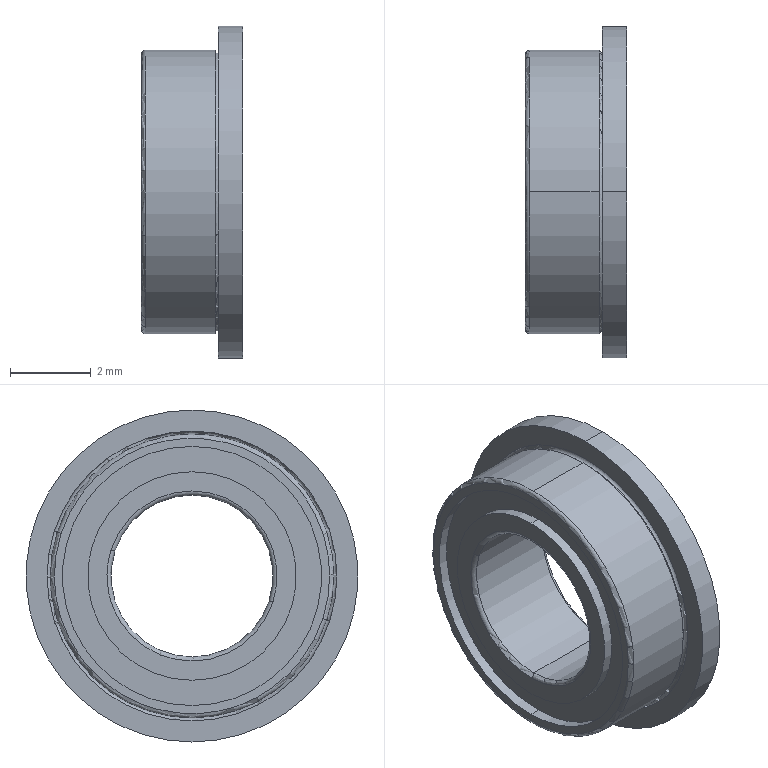Part | NX | features BREP 1 | 1 solid | 31 faces | box 2.5 x 8.2 x 8.2 mm | volume 67.176 mm3 | cylinder 14 | torus 10 | plane 7 | commonest cylinder face diameters 5.15 x4 6.4 x4 4 x2 7 x2 8.2 x2
STEP:
#1=CARTESIAN_POINT('',(1.9,-3.405,-1.106));
#2=VERTEX_POINT('',#1);
#3=CARTESIAN_POINT('',(1.9,-3.253,-1.057));
#4=VERTEX_POINT('',#3);
#5=CARTESIAN_POINT('',(1.9,-3.329,-1.082));
#6=DIRECTION('',(0.,0.309,-0.9511));
#7=DIRECTION('',(-1.,0.,0.));
#8=AXIS2_PLACEMENT_3D('',#5,#6,#7);
#9=CIRCLE('',#8,0.08);
#10=EDGE_CURVE('',#2,#4,#9,.F.);
#11=ORIENTED_EDGE('',*,*,#10,.T.);
#12=CARTESIAN_POINT('',(1.9,3.253,1.057));
#13=VERTEX_POINT('',#12);
#14=CARTESIAN_POINT('',(1.9,0.,0.));
#15=DIRECTION('',(1.,0.,0.));
#16=DIRECTION('',(0.,0.,-1.));
#17=AXIS2_PLACEMENT_3D('',#14,#15,#16);
#18=CIRCLE('',#17,3.42);
#19=EDGE_CURVE('',#4,#13,#18,.T.);
#20=ORIENTED_EDGE('',*,*,#19,.T.);
#21=CARTESIAN_POINT('',(1.9,3.405,1.106));
#22=VERTEX_POINT('',#21);
#23=CARTESIAN_POINT('',(1.9,3.329,1.082));
#24=DIRECTION('',(0.,-0.309,0.9511));
#25=DIRECTION('',(-1.,0.,0.));
#26=AXIS2_PLACEMENT_3D('',#23,#24,#25);
#27=CIRCLE('',#26,0.08);
#28=EDGE_CURVE('',#22,#13,#27,.F.);
#29=ORIENTED_EDGE('',*,*,#28,.F.);
#30=CARTESIAN_POINT('',(1.9,0.,0.));
#31=DIRECTION('',(1.,0.,0.));
#32=DIRECTION('',(0.,-0.9511,-0.309));
#33=AXIS2_PLACEMENT_3D('',#30,#31,#32);
#34=CIRCLE('',#33,3.58);
#35=EDGE_CURVE('',#2,#22,#34,.T.);
#36=ORIENTED_EDGE('',*,*,#35,.F.);
#37=EDGE_LOOP('',(#11,#20,#29,#36));
#38=FACE_BOUND('',#37,.T.);
#39=CARTESIAN_POINT('',(1.9,0.,0.));
#40=DIRECTION('',(1.,0.,0.));
#41=DIRECTION('',(0.,0.309,-0.9511));
#42=AXIS2_PLACEMENT_3D('',#39,#40,#41);
#43=TOROIDAL_SURFACE('',#42,3.5,0.08);
#44=ADVANCED_FACE('',(#38),#43,.F.);
#45=ORIENTED_EDGE('',*,*,#28,.T.);
#46=CARTESIAN_POINT('',(1.9,0.,0.));
#47=DIRECTION('',(1.,0.,0.));
#48=DIRECTION('',(0.,0.,-1.));
#49=AXIS2_PLACEMENT_3D('',#46,#47,#48);
#50=CIRCLE('',#49,3.42);
#51=EDGE_CURVE('',#13,#4,#50,.T.);
#52=ORIENTED_EDGE('',*,*,#51,.T.);
#53=ORIENTED_EDGE('',*,*,#10,.F.);
#54=CARTESIAN_POINT('',(1.9,0.,0.));
#55=DIRECTION('',(1.,0.,0.));
#56=DIRECTION('',(0.,0.,-1.));
#57=AXIS2_PLACEMENT_3D('',#54,#55,#56);
#58=CIRCLE('',#57,3.58);
#59=EDGE_CURVE('',#22,#2,#58,.T.);
#60=ORIENTED_EDGE('',*,*,#59,.F.);
#61=EDGE_LOOP('',(#45,#52,#53,#60));
#62=FACE_BOUND('',#61,.T.);
#63=CARTESIAN_POINT('',(1.9,0.,0.));
#64=DIRECTION('',(1.,0.,0.));
#65=DIRECTION('',(0.,-0.309,0.9511));
#66=AXIS2_PLACEMENT_3D('',#63,#64,#65);
#67=TOROIDAL_SURFACE('',#66,3.5,0.08);
#68=ADVANCED_FACE('',(#62),#67,.F.);
#69=CARTESIAN_POINT('',(0.,0.,2.575));
#70=VERTEX_POINT('',#69);
#71=CARTESIAN_POINT('',(0.,0.,-2.575));
#72=VERTEX_POINT('',#71);
#73=CARTESIAN_POINT('',(0.,0.,0.));
#74=DIRECTION('',(1.,0.,0.));
#75=DIRECTION('',(0.,0.,-1.));
#76=AXIS2_PLACEMENT_3D('',#73,#74,#75);
#77=CIRCLE('',#76,2.575);
#78=EDGE_CURVE('',#70,#72,#77,.T.);
#79=ORIENTED_EDGE('',*,*,#78,.F.);
#80=CARTESIAN_POINT('',(0.,0.,0.));
#81=DIRECTION('',(1.,0.,0.));
#82=DIRECTION('',(0.,0.,-1.));
#83=AXIS2_PLACEMENT_3D('',#80,#81,#82);
#84=CIRCLE('',#83,2.575);
#85=EDGE_CURVE('',#72,#70,#84,.T.);
#86=ORIENTED_EDGE('',*,*,#85,.F.);
#87=EDGE_LOOP('',(#79,#86));
#88=FACE_BOUND('',#87,.T.);
#89=CARTESIAN_POINT('',(0.,1.997,0.6489));
#90=VERTEX_POINT('',#89);
#91=CARTESIAN_POINT('',(0.,-1.997,-0.6489));
#92=VERTEX_POINT('',#91);
#93=CARTESIAN_POINT('',(0.,0.,0.));
#94=DIRECTION('',(1.,0.,0.));
#95=DIRECTION('',(0.,0.,-1.));
#96=AXIS2_PLACEMENT_3D('',#93,#94,#95);
#97=CIRCLE('',#96,2.1);
#98=EDGE_CURVE('',#90,#92,#97,.T.);
#99=ORIENTED_EDGE('',*,*,#98,.T.);
#100=CARTESIAN_POINT('',(0.,-1.997,-0.6489));
#101=CARTESIAN_POINT('',(0.,-1.912,-0.9103));
#102=CARTESIAN_POINT('',(0.,-1.775,-1.155));
#103=CARTESIAN_POINT('',(0.,-1.418,-1.573));
#104=CARTESIAN_POINT('',(0.,-1.198,-1.746));
#105=CARTESIAN_POINT('',(0.,-0.7084,-1.996));
#106=CARTESIAN_POINT('',(0.,-0.4388,-2.072));
#107=CARTESIAN_POINT('',(0.,0.1092,-2.115));
#108=CARTESIAN_POINT('',(0.,0.3874,-2.082));
#109=CARTESIAN_POINT('',(0.,0.9104,-1.912));
#110=CARTESIAN_POINT('',(0.,1.155,-1.775));
#111=CARTESIAN_POINT('',(0.,1.573,-1.418));
#112=CARTESIAN_POINT('',(0.,1.746,-1.198));
#113=CARTESIAN_POINT('',(0.,1.996,-0.7084));
#114=CARTESIAN_POINT('',(0.,2.072,-0.4388));
#115=CARTESIAN_POINT('',(0.,2.115,0.1093));
#116=CARTESIAN_POINT('',(0.,2.082,0.3875));
#117=CARTESIAN_POINT('',(0.,1.997,0.6489));
#118=B_SPLINE_CURVE_WITH_KNOTS('',3,(#100,#101,#102,#103,#104,#105,#106,#107,#108,#109,#110,#111,#112,#113,#114,#115,#116,#117),.UNSPECIFIED.,.F.,.F.,(4,2,2,2,2,2,2,2,4),(0.,0.125,0.25,0.375,0.5,0.625,0.75,0.875,1.),.UNSPECIFIED.);
#119=EDGE_CURVE('',#92,#90,#118,.T.);
#120=ORIENTED_EDGE('',*,*,#119,.T.);
#121=EDGE_LOOP('',(#99,#120));
#122=FACE_BOUND('',#121,.T.);
#123=CARTESIAN_POINT('',(0.,2.575,0.));
#124=DIRECTION('',(-1.,0.,0.));
#125=DIRECTION('',(0.,0.,-1.));
#126=AXIS2_PLACEMENT_3D('',#123,#124,#125);
#127=PLANE('',#126);
#128=ADVANCED_FACE('',(#88,#122),#127,.T.);
#129=CARTESIAN_POINT('',(0.255,0.,2.575));
#130=VERTEX_POINT('',#129);
#131=CARTESIAN_POINT('',(0.,0.,2.575));
#132=DIRECTION('',(1.,0.,0.));
#133=VECTOR('',#132,1000.);
#134=LINE('',#131,#133);
#135=EDGE_CURVE('',#130,#70,#134,.F.);
#136=ORIENTED_EDGE('',*,*,#135,.F.);
#137=CARTESIAN_POINT('',(0.255,0.,-2.575));
#138=VERTEX_POINT('',#137);
#139=CARTESIAN_POINT('',(0.255,0.,0.));
#140=DIRECTION('',(1.,0.,0.));
#141=DIRECTION('',(0.,0.,-1.));
#142=AXIS2_PLACEMENT_3D('',#139,#140,#141);
#143=CIRCLE('',#142,2.575);
#144=EDGE_CURVE('',#138,#130,#143,.T.);
#145=ORIENTED_EDGE('',*,*,#144,.F.);
#146=CARTESIAN_POINT('',(0.,0.,-2.575));
#147=DIRECTION('',(1.,0.,0.));
#148=VECTOR('',#147,1000.);
#149=LINE('',#146,#148);
#150=EDGE_CURVE('',#138,#72,#149,.F.);
#151=ORIENTED_EDGE('',*,*,#150,.T.);
#152=ORIENTED_EDGE('',*,*,#85,.T.);
#153=EDGE_LOOP('',(#136,#145,#151,#152));
#154=FACE_BOUND('',#153,.T.);
#155=CARTESIAN_POINT('',(7.,0.,0.));
#156=DIRECTION('',(1.,0.,0.));
#157=DIRECTION('',(0.,1.,0.));
#158=AXIS2_PLACEMENT_3D('',#155,#156,#157);
#159=CYLINDRICAL_SURFACE('',#158,2.575);
#160=ADVANCED_FACE('',(#154),#159,.T.);
#161=ORIENTED_EDGE('',*,*,#135,.T.);
#162=ORIENTED_EDGE('',*,*,#78,.T.);
#163=ORIENTED_EDGE('',*,*,#150,.F.);
#164=CARTESIAN_POINT('',(0.255,0.,0.));
#165=DIRECTION('',(1.,0.,0.));
#166=DIRECTION('',(0.,0.,-1.));
#167=AXIS2_PLACEMENT_3D('',#164,#165,#166);
#168=CIRCLE('',#167,2.575);
#169=EDGE_CURVE('',#130,#138,#168,.T.);
#170=ORIENTED_EDGE('',*,*,#169,.F.);
#171=EDGE_LOOP('',(#161,#162,#163,#170));
#172=FACE_BOUND('',#171,.T.);
#173=CARTESIAN_POINT('',(7.,0.,0.));
#174=DIRECTION('',(1.,0.,0.));
#175=DIRECTION('',(0.,-1.,0.));
#176=AXIS2_PLACEMENT_3D('',#173,#174,#175);
#177=CYLINDRICAL_SURFACE('',#176,2.575);
#178=ADVANCED_FACE('',(#172),#177,.T.);
#179=CARTESIAN_POINT('',(0.255,0.,3.2));
#180=VERTEX_POINT('',#179);
#181=CARTESIAN_POINT('',(0.255,0.,-3.2));
#182=VERTEX_POINT('',#181);
#183=CARTESIAN_POINT('',(0.255,0.,0.));
#184=DIRECTION('',(1.,0.,0.));
#185=DIRECTION('',(0.,0.,-1.));
#186=AXIS2_PLACEMENT_3D('',#183,#184,#185);
#187=CIRCLE('',#186,3.2);
#188=EDGE_CURVE('',#180,#182,#187,.T.);
#189=ORIENTED_EDGE('',*,*,#188,.F.);
#190=CARTESIAN_POINT('',(0.255,0.,0.));
#191=DIRECTION('',(1.,0.,0.));
#192=DIRECTION('',(0.,0.,-1.));
#193=AXIS2_PLACEMENT_3D('',#190,#191,#192);
#194=CIRCLE('',#193,3.2);
#195=EDGE_CURVE('',#182,#180,#194,.T.);
#196=ORIENTED_EDGE('',*,*,#195,.F.);
#197=EDGE_LOOP('',(#189,#196));
#198=FACE_BOUND('',#197,.T.);
#199=ORIENTED_EDGE('',*,*,#144,.T.);
#200=ORIENTED_EDGE('',*,*,#169,.T.);
#201=EDGE_LOOP('',(#199,#200));
#202=FACE_BOUND('',#201,.T.);
#203=CARTESIAN_POINT('',(0.255,3.2,0.));
#204=DIRECTION('',(-1.,0.,0.));
#205=DIRECTION('',(0.,0.,-1.));
#206=AXIS2_PLACEMENT_3D('',#203,#204,#205);
#207=PLANE('',#206);
#208=ADVANCED_FACE('',(#198,#202),#207,.T.);
#209=CARTESIAN_POINT('',(0.,0.,3.2));
#210=VERTEX_POINT('',#209);
#211=CARTESIAN_POINT('',(0.,0.,3.2));
#212=DIRECTION('',(1.,0.,0.));
#213=VECTOR('',#212,1000.);
#214=LINE('',#211,#213);
#215=EDGE_CURVE('',#210,#180,#214,.T.);
#216=ORIENTED_EDGE('',*,*,#215,.F.);
#217=CARTESIAN_POINT('',(0.,0.,-3.2));
#218=VERTEX_POINT('',#217);
#219=CARTESIAN_POINT('',(0.,0.,0.));
#220=DIRECTION('',(1.,0.,0.));
#221=DIRECTION('',(0.,0.,-1.));
#222=AXIS2_PLACEMENT_3D('',#219,#220,#221);
#223=CIRCLE('',#222,3.2);
#224=EDGE_CURVE('',#218,#210,#223,.T.);
#225=ORIENTED_EDGE('',*,*,#224,.F.);
#226=CARTESIAN_POINT('',(0.,0.,-3.2));
#227=DIRECTION('',(1.,0.,0.));
#228=VECTOR('',#227,1000.);
#229=LINE('',#226,#228);
#230=EDGE_CURVE('',#218,#182,#229,.T.);
#231=ORIENTED_EDGE('',*,*,#230,.T.);
#232=ORIENTED_EDGE('',*,*,#195,.T.);
#233=EDGE_LOOP('',(#216,#225,#231,#232));
#234=FACE_BOUND('',#233,.T.);
#235=CARTESIAN_POINT('',(7.,0.,0.));
#236=DIRECTION('',(1.,0.,0.));
#237=DIRECTION('',(0.,1.,0.));
#238=AXIS2_PLACEMENT_3D('',#235,#236,#237);
#239=CYLINDRICAL_SURFACE('',#238,3.2);
#240=ADVANCED_FACE('',(#234),#239,.F.);
#241=ORIENTED_EDGE('',*,*,#215,.T.);
#242=ORIENTED_EDGE('',*,*,#188,.T.);
#243=ORIENTED_EDGE('',*,*,#230,.F.);
#244=CARTESIAN_POINT('',(0.,0.,0.));
#245=DIRECTION('',(1.,0.,0.));
#246=DIRECTION('',(0.,0.,-1.));
#247=AXIS2_PLACEMENT_3D('',#244,#245,#246);
#248=CIRCLE('',#247,3.2);
#249=EDGE_CURVE('',#210,#218,#248,.T.);
#250=ORIENTED_EDGE('',*,*,#249,.F.);
#251=EDGE_LOOP('',(#241,#242,#243,#250));
#252=FACE_BOUND('',#251,.T.);
#253=CARTESIAN_POINT('',(7.,0.,0.));
#254=DIRECTION('',(1.,0.,0.));
#255=DIRECTION('',(0.,-1.,0.));
#256=AXIS2_PLACEMENT_3D('',#253,#254,#255);
#257=CYLINDRICAL_SURFACE('',#256,3.2);
#258=ADVANCED_FACE('',(#252),#257,.F.);
#259=CARTESIAN_POINT('',(0.,-3.234,-1.051));
#260=VERTEX_POINT('',#259);
#261=CARTESIAN_POINT('',(0.,3.234,1.051));
#262=VERTEX_POINT('',#261);
#263=CARTESIAN_POINT('',(0.,-3.234,-1.051));
#264=CARTESIAN_POINT('',(0.,-3.096,-1.474));
#265=CARTESIAN_POINT('',(0.,-2.874,-1.87));
#266=CARTESIAN_POINT('',(0.,-2.296,-2.547));
#267=CARTESIAN_POINT('',(0.,-1.94,-2.827));
#268=CARTESIAN_POINT('',(0.,-1.147,-3.231));
#269=CARTESIAN_POINT('',(0.,-0.7104,-3.355));
#270=CARTESIAN_POINT('',(0.,0.1769,-3.424));
#271=CARTESIAN_POINT('',(0.,0.6274,-3.371));
#272=CARTESIAN_POINT('',(0.,1.474,-3.096));
#273=CARTESIAN_POINT('',(0.,1.87,-2.874));
#274=CARTESIAN_POINT('',(0.,2.547,-2.296));
#275=CARTESIAN_POINT('',(0.,2.827,-1.94));
#276=CARTESIAN_POINT('',(0.,3.231,-1.147));
#277=CARTESIAN_POINT('',(0.,3.355,-0.7104));
#278=CARTESIAN_POINT('',(0.,3.424,0.1769));
#279=CARTESIAN_POINT('',(0.,3.371,0.6274));
#280=CARTESIAN_POINT('',(0.,3.234,1.051));
#281=B_SPLINE_CURVE_WITH_KNOTS('',3,(#263,#264,#265,#266,#267,#268,#269,#270,#271,#272,#273,#274,#275,#276,#277,#278,#279,#280),.UNSPECIFIED.,.F.,.F.,(4,2,2,2,2,2,2,2,4),(0.,0.125,0.25,0.375,0.5,0.625,0.75,0.875,1.),.UNSPECIFIED.);
#282=EDGE_CURVE('',#260,#262,#281,.T.);
#283=ORIENTED_EDGE('',*,*,#282,.F.);
#284=CARTESIAN_POINT('',(0.,3.234,1.051));
#285=CARTESIAN_POINT('',(0.,3.096,1.474));
#286=CARTESIAN_POINT('',(0.,2.874,1.87));
#287=CARTESIAN_POINT('',(0.,2.296,2.547));
#288=CARTESIAN_POINT('',(0.,1.94,2.827));
#289=CARTESIAN_POINT('',(0.,1.147,3.231));
#290=CARTESIAN_POINT('',(0.,0.7104,3.355));
#291=CARTESIAN_POINT('',(0.,-0.1769,3.424));
#292=CARTESIAN_POINT('',(0.,-0.6274,3.371));
#293=CARTESIAN_POINT('',(0.,-1.474,3.096));
#294=CARTESIAN_POINT('',(0.,-1.87,2.874));
#295=CARTESIAN_POINT('',(0.,-2.547,2.296));
#296=CARTESIAN_POINT('',(0.,-2.827,1.94));
#297=CARTESIAN_POINT('',(0.,-3.231,1.147));
#298=CARTESIAN_POINT('',(0.,-3.355,0.7104));
#299=CARTESIAN_POINT('',(0.,-3.424,-0.1769));
#300=CARTESIAN_POINT('',(0.,-3.371,-0.6274));
#301=CARTESIAN_POINT('',(0.,-3.234,-1.051));
#302=B_SPLINE_CURVE_WITH_KNOTS('',3,(#284,#285,#286,#287,#288,#289,#290,#291,#292,#293,#294,#295,#296,#297,#298,#299,#300,#301),.UNSPECIFIED.,.F.,.F.,(4,2,2,2,2,2,2,2,4),(0.,0.125,0.25,0.375,0.5,0.625,0.75,0.875,1.),.UNSPECIFIED.);
#303=EDGE_CURVE('',#262,#260,#302,.T.);
#304=ORIENTED_EDGE('',*,*,#303,.F.);
#305=EDGE_LOOP('',(#283,#304));
#306=FACE_BOUND('',#305,.T.);
#307=ORIENTED_EDGE('',*,*,#224,.T.);
#308=ORIENTED_EDGE('',*,*,#249,.T.);
#309=EDGE_LOOP('',(#307,#308));
#310=FACE_BOUND('',#309,.T.);
#311=CARTESIAN_POINT('',(0.,3.4,0.));
#312=DIRECTION('',(-1.,0.,0.));
#313=DIRECTION('',(0.,0.,-1.));
#314=AXIS2_PLACEMENT_3D('',#311,#312,#313);
#315=PLANE('',#314);
#316=ADVANCED_FACE('',(#306,#310),#315,.T.);
#317=CARTESIAN_POINT('',(0.1,-3.329,-1.082));
#318=VERTEX_POINT('',#317);
#319=CARTESIAN_POINT('',(0.1,-3.234,-1.051));
#320=DIRECTION('',(0.,0.309,-0.9511));
#321=DIRECTION('',(0.,-0.9511,-0.309));
#322=AXIS2_PLACEMENT_3D('',#319,#320,#321);
#323=CIRCLE('',#322,0.1);
#324=EDGE_CURVE('',#260,#318,#323,.F.);
#325=ORIENTED_EDGE('',*,*,#324,.T.);
#326=CARTESIAN_POINT('',(0.1,0.,3.5));
#327=VERTEX_POINT('',#326);
#328=CARTESIAN_POINT('',(0.1,0.,0.));
#329=DIRECTION('',(1.,0.,0.));
#330=DIRECTION('',(0.,0.,-1.));
#331=AXIS2_PLACEMENT_3D('',#328,#329,#330);
#332=CIRCLE('',#331,3.5);
#333=EDGE_CURVE('',#327,#318,#332,.T.);
#334=ORIENTED_EDGE('',*,*,#333,.F.);
#335=CARTESIAN_POINT('',(0.1,3.329,1.082));
#336=VERTEX_POINT('',#335);
#337=CARTESIAN_POINT('',(0.1,0.,0.));
#338=DIRECTION('',(1.,0.,0.));
#339=DIRECTION('',(0.,0.,-1.));
#340=AXIS2_PLACEMENT_3D('',#337,#338,#339);
#341=CIRCLE('',#340,3.5);
#342=EDGE_CURVE('',#336,#327,#341,.T.);
#343=ORIENTED_EDGE('',*,*,#342,.F.);
#344=CARTESIAN_POINT('',(0.1,3.234,1.051));
#345=DIRECTION('',(0.,-0.309,0.9511));
#346=DIRECTION('',(0.,0.9511,0.309));
#347=AXIS2_PLACEMENT_3D('',#344,#345,#346);
#348=CIRCLE('',#347,0.1);
#349=EDGE_CURVE('',#262,#336,#348,.F.);
#350=ORIENTED_EDGE('',*,*,#349,.F.);
#351=ORIENTED_EDGE('',*,*,#303,.T.);
#352=EDGE_LOOP('',(#325,#334,#343,#350,#351));
#353=FACE_BOUND('',#352,.T.);
#354=CARTESIAN_POINT('',(0.1,0.,0.));
#355=DIRECTION('',(1.,0.,0.));
#356=DIRECTION('',(0.,-0.309,0.9511));
#357=AXIS2_PLACEMENT_3D('',#354,#355,#356);
#358=TOROIDAL_SURFACE('',#357,3.4,0.1);
#359=ADVANCED_FACE('',(#353),#358,.T.);
#360=ORIENTED_EDGE('',*,*,#324,.F.);
#361=ORIENTED_EDGE('',*,*,#282,.T.);
#362=ORIENTED_EDGE('',*,*,#349,.T.);
#363=CARTESIAN_POINT('',(0.1,0.,-3.5));
#364=VERTEX_POINT('',#363);
#365=CARTESIAN_POINT('',(0.1,0.,0.));
#366=DIRECTION('',(1.,0.,0.));
#367=DIRECTION('',(0.,0.,-1.));
#368=AXIS2_PLACEMENT_3D('',#365,#366,#367);
#369=CIRCLE('',#368,3.5);
#370=EDGE_CURVE('',#364,#336,#369,.T.);
#371=ORIENTED_EDGE('',*,*,#370,.F.);
#372=CARTESIAN_POINT('',(0.1,0.,0.));
#373=DIRECTION('',(1.,0.,0.));
#374=DIRECTION('',(0.,0.,-1.));
#375=AXIS2_PLACEMENT_3D('',#372,#373,#374);
#376=CIRCLE('',#375,3.5);
#377=EDGE_CURVE('',#318,#364,#376,.T.);
#378=ORIENTED_EDGE('',*,*,#377,.F.);
#379=EDGE_LOOP('',(#360,#361,#362,#371,#378));
#380=FACE_BOUND('',#379,.T.);
#381=CARTESIAN_POINT('',(0.1,0.,0.));
#382=DIRECTION('',(1.,0.,0.));
#383=DIRECTION('',(0.,0.309,-0.9511));
#384=AXIS2_PLACEMENT_3D('',#381,#382,#383);
#385=TOROIDAL_SURFACE('',#384,3.4,0.1);
#386=ADVANCED_FACE('',(#380),#385,.T.);
#387=CARTESIAN_POINT('',(1.82,0.,3.5));
#388=VERTEX_POINT('',#387);
#389=CARTESIAN_POINT('',(0.1,0.,3.5));
#390=DIRECTION('',(1.,0.,0.));
#391=VECTOR('',#390,1000.);
#392=LINE('',#389,#391);
#393=EDGE_CURVE('',#327,#388,#392,.T.);
#394=ORIENTED_EDGE('',*,*,#393,.F.);
#395=ORIENTED_EDGE('',*,*,#333,.T.);
#396=ORIENTED_EDGE('',*,*,#377,.T.);
#397=CARTESIAN_POINT('',(1.82,0.,-3.5));
#398=VERTEX_POINT('',#397);
#399=CARTESIAN_POINT('',(0.1,0.,-3.5));
#400=DIRECTION('',(1.,0.,0.));
#401=VECTOR('',#400,1000.);
#402=LINE('',#399,#401);
#403=EDGE_CURVE('',#364,#398,#402,.T.);
#404=ORIENTED_EDGE('',*,*,#403,.T.);
#405=CARTESIAN_POINT('',(1.82,-3.329,-1.082));
#406=VERTEX_POINT('',#405);
#407=CARTESIAN_POINT('',(1.82,0.,0.));
#408=DIRECTION('',(1.,0.,0.));
#409=DIRECTION('',(0.,0.,-1.));
#410=AXIS2_PLACEMENT_3D('',#407,#408,#409);
#411=CIRCLE('',#410,3.5);
#412=EDGE_CURVE('',#406,#398,#411,.T.);
#413=ORIENTED_EDGE('',*,*,#412,.F.);
#414=CARTESIAN_POINT('',(1.82,0.,0.));
#415=DIRECTION('',(1.,0.,0.));
#416=DIRECTION('',(0.,0.,-1.));
#417=AXIS2_PLACEMENT_3D('',#414,#415,#416);
#418=CIRCLE('',#417,3.5);
#419=EDGE_CURVE('',#388,#406,#418,.T.);
#420=ORIENTED_EDGE('',*,*,#419,.F.);
#421=EDGE_LOOP('',(#394,#395,#396,#404,#413,#420));
#422=FACE_BOUND('',#421,.T.);
#423=CARTESIAN_POINT('',(7.,0.,0.));
#424=DIRECTION('',(1.,0.,0.));
#425=DIRECTION('',(0.,-1.,0.));
#426=AXIS2_PLACEMENT_3D('',#423,#424,#425);
#427=CYLINDRICAL_SURFACE('',#426,3.5);
#428=ADVANCED_FACE('',(#422),#427,.T.);
#429=ORIENTED_EDGE('',*,*,#51,.F.);
#430=CARTESIAN_POINT('',(1.82,3.329,1.082));
#431=VERTEX_POINT('',#430);
#432=CARTESIAN_POINT('',(1.9,3.329,1.082));
#433=DIRECTION('',(0.,-0.309,0.9511));
#434=DIRECTION('',(-1.,0.,0.));
#435=AXIS2_PLACEMENT_3D('',#432,#433,#434);
#436=CIRCLE('',#435,0.08);
#437=EDGE_CURVE('',#431,#13,#436,.T.);
#438=ORIENTED_EDGE('',*,*,#437,.F.);
#439=CARTESIAN_POINT('',(1.82,0.,0.));
#440=DIRECTION('',(1.,0.,0.));
#441=DIRECTION('',(0.,0.,-1.));
#442=AXIS2_PLACEMENT_3D('',#439,#440,#441);
#443=CIRCLE('',#442,3.5);
#444=EDGE_CURVE('',#431,#388,#443,.T.);
#445=ORIENTED_EDGE('',*,*,#444,.T.);
#446=ORIENTED_EDGE('',*,*,#419,.T.);
#447=CARTESIAN_POINT('',(1.9,-3.329,-1.082));
#448=DIRECTION('',(0.,0.309,-0.9511));
#449=DIRECTION('',(-1.,0.,0.));
#450=AXIS2_PLACEMENT_3D('',#447,#448,#449);
#451=CIRCLE('',#450,0.08);
#452=EDGE_CURVE('',#406,#4,#451,.T.);
#453=ORIENTED_EDGE('',*,*,#452,.T.);
#454=EDGE_LOOP('',(#429,#438,#445,#446,#453));
#455=FACE_BOUND('',#454,.T.);
#456=CARTESIAN_POINT('',(1.9,0.,0.));
#457=DIRECTION('',(1.,0.,0.));
#458=DIRECTION('',(0.,-0.309,0.9511));
#459=AXIS2_PLACEMENT_3D('',#456,#457,#458);
#460=TOROIDAL_SURFACE('',#459,3.5,0.08);
#461=ADVANCED_FACE('',(#455),#460,.F.);
#462=ORIENTED_EDGE('',*,*,#393,.T.);
#463=ORIENTED_EDGE('',*,*,#444,.F.);
#464=CARTESIAN_POINT('',(1.82,0.,0.));
#465=DIRECTION('',(1.,0.,0.));
#466=DIRECTION('',(0.,0.,-1.));
#467=AXIS2_PLACEMENT_3D('',#464,#465,#466);
#468=CIRCLE('',#467,3.5);
#469=EDGE_CURVE('',#398,#431,#468,.T.);
#470=ORIENTED_EDGE('',*,*,#469,.F.);
#471=ORIENTED_EDGE('',*,*,#403,.F.);
#472=ORIENTED_EDGE('',*,*,#370,.T.);
#473=ORIENTED_EDGE('',*,*,#342,.T.);
#474=EDGE_LOOP('',(#462,#463,#470,#471,#472,#473));
#475=FACE_BOUND('',#474,.T.);
#476=CARTESIAN_POINT('',(7.,0.,0.));
#477=DIRECTION('',(1.,0.,0.));
#478=DIRECTION('',(0.,1.,0.));
#479=AXIS2_PLACEMENT_3D('',#476,#477,#478);
#480=CYLINDRICAL_SURFACE('',#479,3.5);
#481=ADVANCED_FACE('',(#475),#480,.T.);
#482=ORIENTED_EDGE('',*,*,#19,.F.);
#483=ORIENTED_EDGE('',*,*,#452,.F.);
#484=ORIENTED_EDGE('',*,*,#412,.T.);
#485=ORIENTED_EDGE('',*,*,#469,.T.);
#486=ORIENTED_EDGE('',*,*,#437,.T.);
#487=EDGE_LOOP('',(#482,#483,#484,#485,#486));
#488=FACE_BOUND('',#487,.T.);
#489=CARTESIAN_POINT('',(1.9,0.,0.));
#490=DIRECTION('',(1.,0.,0.));
#491=DIRECTION('',(0.,0.309,-0.9511));
#492=AXIS2_PLACEMENT_3D('',#489,#490,#491);
#493=TOROIDAL_SURFACE('',#492,3.5,0.08);
#494=ADVANCED_FACE('',(#488),#493,.F.);
#495=CARTESIAN_POINT('',(1.9,0.,4.1));
#496=VERTEX_POINT('',#495);
#497=CARTESIAN_POINT('',(1.9,0.,-4.1));
#498=VERTEX_POINT('',#497);
#499=CARTESIAN_POINT('',(1.9,0.,0.));
#500=DIRECTION('',(1.,0.,0.));
#501=DIRECTION('',(0.,0.,-1.));
#502=AXIS2_PLACEMENT_3D('',#499,#500,#501);
#503=CIRCLE('',#502,4.1);
#504=EDGE_CURVE('',#496,#498,#503,.T.);
#505=ORIENTED_EDGE('',*,*,#504,.F.);
#506=CARTESIAN_POINT('',(1.9,0.,0.));
#507=DIRECTION('',(1.,0.,0.));
#508=DIRECTION('',(0.,0.,-1.));
#509=AXIS2_PLACEMENT_3D('',#506,#507,#508);
#510=CIRCLE('',#509,4.1);
#511=EDGE_CURVE('',#498,#496,#510,.T.);
#512=ORIENTED_EDGE('',*,*,#511,.F.);
#513=EDGE_LOOP('',(#505,#512));
#514=FACE_BOUND('',#513,.T.);
#515=ORIENTED_EDGE('',*,*,#59,.T.);
#516=ORIENTED_EDGE('',*,*,#35,.T.);
#517=EDGE_LOOP('',(#515,#516));
#518=FACE_BOUND('',#517,.T.);
#519=CARTESIAN_POINT('',(1.9,4.1,0.));
#520=DIRECTION('',(-1.,0.,0.));
#521=DIRECTION('',(0.,0.,-1.));
#522=AXIS2_PLACEMENT_3D('',#519,#520,#521);
#523=PLANE('',#522);
#524=ADVANCED_FACE('',(#514,#518),#523,.T.);
#525=CARTESIAN_POINT('',(2.5,0.,4.1));
#526=VERTEX_POINT('',#525);
#527=CARTESIAN_POINT('',(1.9,0.,4.1));
#528=DIRECTION('',(1.,0.,0.));
#529=VECTOR('',#528,1000.);
#530=LINE('',#527,#529);
#531=EDGE_CURVE('',#526,#496,#530,.F.);
#532=ORIENTED_EDGE('',*,*,#531,.F.);
#533=CARTESIAN_POINT('',(2.5,0.,-4.1));
#534=VERTEX_POINT('',#533);
#535=CARTESIAN_POINT('',(2.5,0.,0.));
#536=DIRECTION('',(1.,0.,0.));
#537=DIRECTION('',(0.,0.,-1.));
#538=AXIS2_PLACEMENT_3D('',#535,#536,#537);
#539=CIRCLE('',#538,4.1);
#540=EDGE_CURVE('',#534,#526,#539,.T.);
#541=ORIENTED_EDGE('',*,*,#540,.F.);
#542=CARTESIAN_POINT('',(1.9,0.,-4.1));
#543=DIRECTION('',(1.,0.,0.));
#544=VECTOR('',#543,1000.);
#545=LINE('',#542,#544);
#546=EDGE_CURVE('',#534,#498,#545,.F.);
#547=ORIENTED_EDGE('',*,*,#546,.T.);
#548=ORIENTED_EDGE('',*,*,#511,.T.);
#549=EDGE_LOOP('',(#532,#541,#547,#548));
#550=FACE_BOUND('',#549,.T.);
#551=CARTESIAN_POINT('',(7.,0.,0.));
#552=DIRECTION('',(1.,0.,0.));
#553=DIRECTION('',(0.,1.,0.));
#554=AXIS2_PLACEMENT_3D('',#551,#552,#553);
#555=CYLINDRICAL_SURFACE('',#554,4.1);
#556=ADVANCED_FACE('',(#550),#555,.T.);
#557=ORIENTED_EDGE('',*,*,#531,.T.);
#558=ORIENTED_EDGE('',*,*,#504,.T.);
#559=ORIENTED_EDGE('',*,*,#546,.F.);
#560=CARTESIAN_POINT('',(2.5,0.,0.));
#561=DIRECTION('',(1.,0.,0.));
#562=DIRECTION('',(0.,0.,-1.));
#563=AXIS2_PLACEMENT_3D('',#560,#561,#562);
#564=CIRCLE('',#563,4.1);
#565=EDGE_CURVE('',#526,#534,#564,.T.);
#566=ORIENTED_EDGE('',*,*,#565,.F.);
#567=EDGE_LOOP('',(#557,#558,#559,#566));
#568=FACE_BOUND('',#567,.T.);
#569=CARTESIAN_POINT('',(7.,0.,0.));
#570=DIRECTION('',(1.,0.,0.));
#571=DIRECTION('',(0.,-1.,0.));
#572=AXIS2_PLACEMENT_3D('',#569,#570,#571);
#573=CYLINDRICAL_SURFACE('',#572,4.1);
#574=ADVANCED_FACE('',(#568),#573,.T.);
#575=ORIENTED_EDGE('',*,*,#540,.T.);
#576=ORIENTED_EDGE('',*,*,#565,.T.);
#577=EDGE_LOOP('',(#575,#576));
#578=FACE_BOUND('',#577,.T.);
#579=CARTESIAN_POINT('',(2.5,0.,3.2));
#580=VERTEX_POINT('',#579);
#581=CARTESIAN_POINT('',(2.5,0.,-3.2));
#582=VERTEX_POINT('',#581);
#583=CARTESIAN_POINT('',(2.5,0.,0.));
#584=DIRECTION('',(1.,0.,0.));
#585=DIRECTION('',(0.,0.,-1.));
#586=AXIS2_PLACEMENT_3D('',#583,#584,#585);
#587=CIRCLE('',#586,3.2);
#588=EDGE_CURVE('',#580,#582,#587,.T.);
#589=ORIENTED_EDGE('',*,*,#588,.F.);
#590=CARTESIAN_POINT('',(2.5,0.,0.));
#591=DIRECTION('',(1.,0.,0.));
#592=DIRECTION('',(0.,0.,-1.));
#593=AXIS2_PLACEMENT_3D('',#590,#591,#592);
#594=CIRCLE('',#593,3.2);
#595=EDGE_CURVE('',#582,#580,#594,.T.);
#596=ORIENTED_EDGE('',*,*,#595,.F.);
#597=EDGE_LOOP('',(#589,#596));
#598=FACE_BOUND('',#597,.T.);
#599=CARTESIAN_POINT('',(2.5,3.2,0.));
#600=DIRECTION('',(1.,0.,0.));
#601=DIRECTION('',(0.,-1.,0.));
#602=AXIS2_PLACEMENT_3D('',#599,#600,#601);
#603=PLANE('',#602);
#604=ADVANCED_FACE('',(#578,#598),#603,.T.);
#605=CARTESIAN_POINT('',(2.245,0.,3.2));
#606=VERTEX_POINT('',#605);
#607=CARTESIAN_POINT('',(2.245,0.,3.2));
#608=DIRECTION('',(1.,0.,0.));
#609=VECTOR('',#608,1000.);
#610=LINE('',#607,#609);
#611=EDGE_CURVE('',#606,#580,#610,.T.);
#612=ORIENTED_EDGE('',*,*,#611,.F.);
#613=CARTESIAN_POINT('',(2.245,0.,-3.2));
#614=VERTEX_POINT('',#613);
#615=CARTESIAN_POINT('',(2.245,0.,0.));
#616=DIRECTION('',(1.,0.,0.));
#617=DIRECTION('',(0.,0.,-1.));
#618=AXIS2_PLACEMENT_3D('',#615,#616,#617);
#619=CIRCLE('',#618,3.2);
#620=EDGE_CURVE('',#614,#606,#619,.T.);
#621=ORIENTED_EDGE('',*,*,#620,.F.);
#622=CARTESIAN_POINT('',(2.245,0.,-3.2));
#623=DIRECTION('',(1.,0.,0.));
#624=VECTOR('',#623,1000.);
#625=LINE('',#622,#624);
#626=EDGE_CURVE('',#614,#582,#625,.T.);
#627=ORIENTED_EDGE('',*,*,#626,.T.);
#628=ORIENTED_EDGE('',*,*,#595,.T.);
#629=EDGE_LOOP('',(#612,#621,#627,#628));
#630=FACE_BOUND('',#629,.T.);
#631=CARTESIAN_POINT('',(7.,0.,0.));
#632=DIRECTION('',(1.,0.,0.));
#633=DIRECTION('',(0.,1.,0.));
#634=AXIS2_PLACEMENT_3D('',#631,#632,#633);
#635=CYLINDRICAL_SURFACE('',#634,3.2);
#636=ADVANCED_FACE('',(#630),#635,.F.);
#637=ORIENTED_EDGE('',*,*,#611,.T.);
#638=ORIENTED_EDGE('',*,*,#588,.T.);
#639=ORIENTED_EDGE('',*,*,#626,.F.);
#640=CARTESIAN_POINT('',(2.245,0.,0.));
#641=DIRECTION('',(1.,0.,0.));
#642=DIRECTION('',(0.,0.,-1.));
#643=AXIS2_PLACEMENT_3D('',#640,#641,#642);
#644=CIRCLE('',#643,3.2);
#645=EDGE_CURVE('',#606,#614,#644,.T.);
#646=ORIENTED_EDGE('',*,*,#645,.F.);
#647=EDGE_LOOP('',(#637,#638,#639,#646));
#648=FACE_BOUND('',#647,.T.);
#649=CARTESIAN_POINT('',(7.,0.,0.));
#650=DIRECTION('',(1.,0.,0.));
#651=DIRECTION('',(0.,-1.,0.));
#652=AXIS2_PLACEMENT_3D('',#649,#650,#651);
#653=CYLINDRICAL_SURFACE('',#652,3.2);
#654=ADVANCED_FACE('',(#648),#653,.F.);
#655=ORIENTED_EDGE('',*,*,#620,.T.);
#656=ORIENTED_EDGE('',*,*,#645,.T.);
#657=EDGE_LOOP('',(#655,#656));
#658=FACE_BOUND('',#657,.T.);
#659=CARTESIAN_POINT('',(2.245,0.,2.575));
#660=VERTEX_POINT('',#659);
#661=CARTESIAN_POINT('',(2.245,0.,-2.575));
#662=VERTEX_POINT('',#661);
#663=CARTESIAN_POINT('',(2.245,0.,0.));
#664=DIRECTION('',(1.,0.,0.));
#665=DIRECTION('',(0.,0.,-1.));
#666=AXIS2_PLACEMENT_3D('',#663,#664,#665);
#667=CIRCLE('',#666,2.575);
#668=EDGE_CURVE('',#660,#662,#667,.T.);
#669=ORIENTED_EDGE('',*,*,#668,.F.);
#670=CARTESIAN_POINT('',(2.245,0.,0.));
#671=DIRECTION('',(1.,0.,0.));
#672=DIRECTION('',(0.,0.,-1.));
#673=AXIS2_PLACEMENT_3D('',#670,#671,#672);
#674=CIRCLE('',#673,2.575);
#675=EDGE_CURVE('',#662,#660,#674,.T.);
#676=ORIENTED_EDGE('',*,*,#675,.F.);
#677=EDGE_LOOP('',(#669,#676));
#678=FACE_BOUND('',#677,.T.);
#679=CARTESIAN_POINT('',(2.245,2.575,0.));
#680=DIRECTION('',(1.,0.,0.));
#681=DIRECTION('',(0.,-1.,0.));
#682=AXIS2_PLACEMENT_3D('',#679,#680,#681);
#683=PLANE('',#682);
#684=ADVANCED_FACE('',(#658,#678),#683,.T.);
#685=CARTESIAN_POINT('',(2.5,0.,2.575));
#686=VERTEX_POINT('',#685);
#687=CARTESIAN_POINT('',(2.245,0.,2.575));
#688=DIRECTION('',(1.,0.,0.));
#689=VECTOR('',#688,1000.);
#690=LINE('',#687,#689);
#691=EDGE_CURVE('',#686,#660,#690,.F.);
#692=ORIENTED_EDGE('',*,*,#691,.F.);
#693=CARTESIAN_POINT('',(2.5,0.,-2.575));
#694=VERTEX_POINT('',#693);
#695=CARTESIAN_POINT('',(2.5,0.,0.));
#696=DIRECTION('',(1.,0.,0.));
#697=DIRECTION('',(0.,0.,-1.));
#698=AXIS2_PLACEMENT_3D('',#695,#696,#697);
#699=CIRCLE('',#698,2.575);
#700=EDGE_CURVE('',#694,#686,#699,.T.);
#701=ORIENTED_EDGE('',*,*,#700,.F.);
#702=CARTESIAN_POINT('',(2.245,0.,-2.575));
#703=DIRECTION('',(1.,0.,0.));
#704=VECTOR('',#703,1000.);
#705=LINE('',#702,#704);
#706=EDGE_CURVE('',#694,#662,#705,.F.);
#707=ORIENTED_EDGE('',*,*,#706,.T.);
#708=ORIENTED_EDGE('',*,*,#675,.T.);
#709=EDGE_LOOP('',(#692,#701,#707,#708));
#710=FACE_BOUND('',#709,.T.);
#711=CARTESIAN_POINT('',(7.,0.,0.));
#712=DIRECTION('',(1.,0.,0.));
#713=DIRECTION('',(0.,1.,0.));
#714=AXIS2_PLACEMENT_3D('',#711,#712,#713);
#715=CYLINDRICAL_SURFACE('',#714,2.575);
#716=ADVANCED_FACE('',(#710),#715,.T.);
#717=ORIENTED_EDGE('',*,*,#691,.T.);
#718=ORIENTED_EDGE('',*,*,#668,.T.);
#719=ORIENTED_EDGE('',*,*,#706,.F.);
#720=CARTESIAN_POINT('',(2.5,0.,0.));
#721=DIRECTION('',(1.,0.,0.));
#722=DIRECTION('',(0.,0.,-1.));
#723=AXIS2_PLACEMENT_3D('',#720,#721,#722);
#724=CIRCLE('',#723,2.575);
#725=EDGE_CURVE('',#686,#694,#724,.T.);
#726=ORIENTED_EDGE('',*,*,#725,.F.);
#727=EDGE_LOOP('',(#717,#718,#719,#726));
#728=FACE_BOUND('',#727,.T.);
#729=CARTESIAN_POINT('',(7.,0.,0.));
#730=DIRECTION('',(1.,0.,0.));
#731=DIRECTION('',(0.,-1.,0.));
#732=AXIS2_PLACEMENT_3D('',#729,#730,#731);
#733=CYLINDRICAL_SURFACE('',#732,2.575);
#734=ADVANCED_FACE('',(#728),#733,.T.);
#735=ORIENTED_EDGE('',*,*,#700,.T.);
#736=ORIENTED_EDGE('',*,*,#725,.T.);
#737=EDGE_LOOP('',(#735,#736));
#738=FACE_BOUND('',#737,.T.);
#739=CARTESIAN_POINT('',(2.5,-1.997,-0.6489));
#740=VERTEX_POINT('',#739);
#741=CARTESIAN_POINT('',(2.5,1.997,0.6489));
#742=VERTEX_POINT('',#741);
#743=CARTESIAN_POINT('',(2.5,-1.997,-0.6489));
#744=CARTESIAN_POINT('',(2.5,-1.912,-0.9104));
#745=CARTESIAN_POINT('',(2.5,-1.775,-1.155));
#746=CARTESIAN_POINT('',(2.5,-1.418,-1.573));
#747=CARTESIAN_POINT('',(2.5,-1.198,-1.746));
#748=CARTESIAN_POINT('',(2.5,-0.7085,-1.996));
#749=CARTESIAN_POINT('',(2.5,-0.4388,-2.072));
#750=CARTESIAN_POINT('',(2.5,0.1093,-2.115));
#751=CARTESIAN_POINT('',(2.5,0.3875,-2.082));
#752=CARTESIAN_POINT('',(2.5,0.9104,-1.912));
#753=CARTESIAN_POINT('',(2.5,1.155,-1.775));
#754=CARTESIAN_POINT('',(2.5,1.573,-1.418));
#755=CARTESIAN_POINT('',(2.5,1.746,-1.198));
#756=CARTESIAN_POINT('',(2.5,1.996,-0.7085));
#757=CARTESIAN_POINT('',(2.5,2.072,-0.4388));
#758=CARTESIAN_POINT('',(2.5,2.115,0.1093));
#759=CARTESIAN_POINT('',(2.5,2.082,0.3875));
#760=CARTESIAN_POINT('',(2.5,1.997,0.6489));
#761=B_SPLINE_CURVE_WITH_KNOTS('',3,(#743,#744,#745,#746,#747,#748,#749,#750,#751,#752,#753,#754,#755,#756,#757,#758,#759,#760),.UNSPECIFIED.,.F.,.F.,(4,2,2,2,2,2,2,2,4),(0.,0.125,0.25,0.375,0.5,0.625,0.75,0.875,1.),.UNSPECIFIED.);
#762=EDGE_CURVE('',#740,#742,#761,.T.);
#763=ORIENTED_EDGE('',*,*,#762,.F.);
#764=CARTESIAN_POINT('',(2.5,1.997,0.6489));
#765=CARTESIAN_POINT('',(2.5,1.912,0.9104));
#766=CARTESIAN_POINT('',(2.5,1.775,1.155));
#767=CARTESIAN_POINT('',(2.5,1.418,1.573));
#768=CARTESIAN_POINT('',(2.5,1.198,1.746));
#769=CARTESIAN_POINT('',(2.5,0.7085,1.996));
#770=CARTESIAN_POINT('',(2.5,0.4388,2.072));
#771=CARTESIAN_POINT('',(2.5,-0.1093,2.115));
#772=CARTESIAN_POINT('',(2.5,-0.3875,2.082));
#773=CARTESIAN_POINT('',(2.5,-0.9104,1.912));
#774=CARTESIAN_POINT('',(2.5,-1.155,1.775));
#775=CARTESIAN_POINT('',(2.5,-1.573,1.418));
#776=CARTESIAN_POINT('',(2.5,-1.746,1.198));
#777=CARTESIAN_POINT('',(2.5,-1.996,0.7085));
#778=CARTESIAN_POINT('',(2.5,-2.072,0.4388));
#779=CARTESIAN_POINT('',(2.5,-2.115,-0.1093));
#780=CARTESIAN_POINT('',(2.5,-2.082,-0.3875));
#781=CARTESIAN_POINT('',(2.5,-1.997,-0.6489));
#782=B_SPLINE_CURVE_WITH_KNOTS('',3,(#764,#765,#766,#767,#768,#769,#770,#771,#772,#773,#774,#775,#776,#777,#778,#779,#780,#781),.UNSPECIFIED.,.F.,.F.,(4,2,2,2,2,2,2,2,4),(0.,0.125,0.25,0.375,0.5,0.625,0.75,0.875,1.),.UNSPECIFIED.);
#783=EDGE_CURVE('',#742,#740,#782,.T.);
#784=ORIENTED_EDGE('',*,*,#783,.F.);
#785=EDGE_LOOP('',(#763,#784));
#786=FACE_BOUND('',#785,.T.);
#787=CARTESIAN_POINT('',(2.5,2.1,0.));
#788=DIRECTION('',(1.,0.,0.));
#789=DIRECTION('',(0.,-1.,0.));
#790=AXIS2_PLACEMENT_3D('',#787,#788,#789);
#791=PLANE('',#790);
#792=ADVANCED_FACE('',(#738,#786),#791,.T.);
#793=CARTESIAN_POINT('',(2.4,-1.902,-0.618));
#794=VERTEX_POINT('',#793);
#795=CARTESIAN_POINT('',(2.4,-1.997,-0.6489));
#796=DIRECTION('',(0.,0.309,-0.9511));
#797=DIRECTION('',(0.,0.9511,0.309));
#798=AXIS2_PLACEMENT_3D('',#795,#796,#797);
#799=CIRCLE('',#798,0.1);
#800=EDGE_CURVE('',#740,#794,#799,.F.);
#801=ORIENTED_EDGE('',*,*,#800,.T.);
#802=CARTESIAN_POINT('',(2.4,0.,2.));
#803=VERTEX_POINT('',#802);
#804=CARTESIAN_POINT('',(2.4,0.,0.));
#805=DIRECTION('',(1.,0.,0.));
#806=DIRECTION('',(0.,0.,-1.));
#807=AXIS2_PLACEMENT_3D('',#804,#805,#806);
#808=CIRCLE('',#807,2.);
#809=EDGE_CURVE('',#803,#794,#808,.T.);
#810=ORIENTED_EDGE('',*,*,#809,.F.);
#811=CARTESIAN_POINT('',(2.4,1.902,0.618));
#812=VERTEX_POINT('',#811);
#813=CARTESIAN_POINT('',(2.4,0.,0.));
#814=DIRECTION('',(1.,0.,0.));
#815=DIRECTION('',(0.,0.,-1.));
#816=AXIS2_PLACEMENT_3D('',#813,#814,#815);
#817=CIRCLE('',#816,2.);
#818=EDGE_CURVE('',#812,#803,#817,.T.);
#819=ORIENTED_EDGE('',*,*,#818,.F.);
#820=CARTESIAN_POINT('',(2.4,1.997,0.6489));
#821=DIRECTION('',(0.,-0.309,0.9511));
#822=DIRECTION('',(0.,-0.9511,-0.309));
#823=AXIS2_PLACEMENT_3D('',#820,#821,#822);
#824=CIRCLE('',#823,0.1);
#825=EDGE_CURVE('',#742,#812,#824,.F.);
#826=ORIENTED_EDGE('',*,*,#825,.F.);
#827=ORIENTED_EDGE('',*,*,#783,.T.);
#828=EDGE_LOOP('',(#801,#810,#819,#826,#827));
#829=FACE_BOUND('',#828,.T.);
#830=CARTESIAN_POINT('',(2.4,0.,0.));
#831=DIRECTION('',(1.,0.,0.));
#832=DIRECTION('',(0.,-0.309,0.9511));
#833=AXIS2_PLACEMENT_3D('',#830,#831,#832);
#834=TOROIDAL_SURFACE('',#833,2.1,0.1);
#835=ADVANCED_FACE('',(#829),#834,.T.);
#836=ORIENTED_EDGE('',*,*,#800,.F.);
#837=ORIENTED_EDGE('',*,*,#762,.T.);
#838=ORIENTED_EDGE('',*,*,#825,.T.);
#839=CARTESIAN_POINT('',(2.4,0.,-2.));
#840=VERTEX_POINT('',#839);
#841=CARTESIAN_POINT('',(2.4,0.,0.));
#842=DIRECTION('',(1.,0.,0.));
#843=DIRECTION('',(0.,0.,-1.));
#844=AXIS2_PLACEMENT_3D('',#841,#842,#843);
#845=CIRCLE('',#844,2.);
#846=EDGE_CURVE('',#840,#812,#845,.T.);
#847=ORIENTED_EDGE('',*,*,#846,.F.);
#848=CARTESIAN_POINT('',(2.4,0.,0.));
#849=DIRECTION('',(1.,0.,0.));
#850=DIRECTION('',(0.,0.,-1.));
#851=AXIS2_PLACEMENT_3D('',#848,#849,#850);
#852=CIRCLE('',#851,2.);
#853=EDGE_CURVE('',#794,#840,#852,.T.);
#854=ORIENTED_EDGE('',*,*,#853,.F.);
#855=EDGE_LOOP('',(#836,#837,#838,#847,#854));
#856=FACE_BOUND('',#855,.T.);
#857=CARTESIAN_POINT('',(2.4,0.,0.));
#858=DIRECTION('',(1.,0.,0.));
#859=DIRECTION('',(0.,0.309,-0.9511));
#860=AXIS2_PLACEMENT_3D('',#857,#858,#859);
#861=TOROIDAL_SURFACE('',#860,2.1,0.1);
#862=ADVANCED_FACE('',(#856),#861,.T.);
#863=CARTESIAN_POINT('',(0.1,0.,2.));
#864=VERTEX_POINT('',#863);
#865=CARTESIAN_POINT('',(0.1,0.,2.));
#866=DIRECTION('',(1.,0.,0.));
#867=VECTOR('',#866,1000.);
#868=LINE('',#865,#867);
#869=EDGE_CURVE('',#803,#864,#868,.F.);
#870=ORIENTED_EDGE('',*,*,#869,.F.);
#871=ORIENTED_EDGE('',*,*,#809,.T.);
#872=ORIENTED_EDGE('',*,*,#853,.T.);
#873=CARTESIAN_POINT('',(0.1,0.,-2.));
#874=VERTEX_POINT('',#873);
#875=CARTESIAN_POINT('',(0.1,0.,-2.));
#876=DIRECTION('',(1.,0.,0.));
#877=VECTOR('',#876,1000.);
#878=LINE('',#875,#877);
#879=EDGE_CURVE('',#840,#874,#878,.F.);
#880=ORIENTED_EDGE('',*,*,#879,.T.);
#881=CARTESIAN_POINT('',(0.1,-1.902,-0.618));
#882=VERTEX_POINT('',#881);
#883=CARTESIAN_POINT('',(0.1,0.,0.));
#884=DIRECTION('',(1.,0.,0.));
#885=DIRECTION('',(0.,0.,-1.));
#886=AXIS2_PLACEMENT_3D('',#883,#884,#885);
#887=CIRCLE('',#886,2.);
#888=EDGE_CURVE('',#882,#874,#887,.T.);
#889=ORIENTED_EDGE('',*,*,#888,.F.);
#890=CARTESIAN_POINT('',(0.1,0.,0.));
#891=DIRECTION('',(1.,0.,0.));
#892=DIRECTION('',(0.,0.,-1.));
#893=AXIS2_PLACEMENT_3D('',#890,#891,#892);
#894=CIRCLE('',#893,2.);
#895=EDGE_CURVE('',#864,#882,#894,.T.);
#896=ORIENTED_EDGE('',*,*,#895,.F.);
#897=EDGE_LOOP('',(#870,#871,#872,#880,#889,#896));
#898=FACE_BOUND('',#897,.T.);
#899=CARTESIAN_POINT('',(7.,0.,0.));
#900=DIRECTION('',(1.,0.,0.));
#901=DIRECTION('',(0.,-1.,0.));
#902=AXIS2_PLACEMENT_3D('',#899,#900,#901);
#903=CYLINDRICAL_SURFACE('',#902,2.);
#904=ADVANCED_FACE('',(#898),#903,.F.);
#905=CARTESIAN_POINT('',(0.1,-1.997,-0.6489));
#906=DIRECTION('',(0.,0.309,-0.9511));
#907=DIRECTION('',(-1.,0.,0.));
#908=AXIS2_PLACEMENT_3D('',#905,#906,#907);
#909=CIRCLE('',#908,0.1);
#910=EDGE_CURVE('',#882,#92,#909,.F.);
#911=ORIENTED_EDGE('',*,*,#910,.T.);
#912=ORIENTED_EDGE('',*,*,#98,.F.);
#913=CARTESIAN_POINT('',(0.1,1.902,0.618));
#914=VERTEX_POINT('',#913);
#915=CARTESIAN_POINT('',(0.1,1.997,0.6489));
#916=DIRECTION('',(0.,-0.309,0.9511));
#917=DIRECTION('',(-1.,0.,0.));
#918=AXIS2_PLACEMENT_3D('',#915,#916,#917);
#919=CIRCLE('',#918,0.1);
#920=EDGE_CURVE('',#914,#90,#919,.F.);
#921=ORIENTED_EDGE('',*,*,#920,.F.);
#922=CARTESIAN_POINT('',(0.1,0.,0.));
#923=DIRECTION('',(1.,0.,0.));
#924=DIRECTION('',(0.,0.,-1.));
#925=AXIS2_PLACEMENT_3D('',#922,#923,#924);
#926=CIRCLE('',#925,2.);
#927=EDGE_CURVE('',#914,#864,#926,.T.);
#928=ORIENTED_EDGE('',*,*,#927,.T.);
#929=ORIENTED_EDGE('',*,*,#895,.T.);
#930=EDGE_LOOP('',(#911,#912,#921,#928,#929));
#931=FACE_BOUND('',#930,.T.);
#932=CARTESIAN_POINT('',(0.1,0.,0.));
#933=DIRECTION('',(1.,0.,0.));
#934=DIRECTION('',(0.,-0.309,0.9511));
#935=AXIS2_PLACEMENT_3D('',#932,#933,#934);
#936=TOROIDAL_SURFACE('',#935,2.1,0.1);
#937=ADVANCED_FACE('',(#931),#936,.T.);
#938=ORIENTED_EDGE('',*,*,#869,.T.);
#939=ORIENTED_EDGE('',*,*,#927,.F.);
#940=CARTESIAN_POINT('',(0.1,0.,0.));
#941=DIRECTION('',(1.,0.,0.));
#942=DIRECTION('',(0.,0.,-1.));
#943=AXIS2_PLACEMENT_3D('',#940,#941,#942);
#944=CIRCLE('',#943,2.);
#945=EDGE_CURVE('',#874,#914,#944,.T.);
#946=ORIENTED_EDGE('',*,*,#945,.F.);
#947=ORIENTED_EDGE('',*,*,#879,.F.);
#948=ORIENTED_EDGE('',*,*,#846,.T.);
#949=ORIENTED_EDGE('',*,*,#818,.T.);
#950=EDGE_LOOP('',(#938,#939,#946,#947,#948,#949));
#951=FACE_BOUND('',#950,.T.);
#952=CARTESIAN_POINT('',(7.,0.,0.));
#953=DIRECTION('',(1.,0.,0.));
#954=DIRECTION('',(0.,1.,0.));
#955=AXIS2_PLACEMENT_3D('',#952,#953,#954);
#956=CYLINDRICAL_SURFACE('',#955,2.);
#957=ADVANCED_FACE('',(#951),#956,.F.);
#958=ORIENTED_EDGE('',*,*,#910,.F.);
#959=ORIENTED_EDGE('',*,*,#888,.T.);
#960=ORIENTED_EDGE('',*,*,#945,.T.);
#961=ORIENTED_EDGE('',*,*,#920,.T.);
#962=ORIENTED_EDGE('',*,*,#119,.F.);
#963=EDGE_LOOP('',(#958,#959,#960,#961,#962));
#964=FACE_BOUND('',#963,.T.);
#965=CARTESIAN_POINT('',(0.1,0.,0.));
#966=DIRECTION('',(1.,0.,0.));
#967=DIRECTION('',(0.,0.309,-0.9511));
#968=AXIS2_PLACEMENT_3D('',#965,#966,#967);
#969=TOROIDAL_SURFACE('',#968,2.1,0.1);
#970=ADVANCED_FACE('',(#964),#969,.T.);
#971=CLOSED_SHELL('',(#44,#68,#128,#160,#178,#208,#240,#258,#316,#359,#386,#428,#461,#481,#494,#524,#556,#574,#604,#636,#654,#684,#716,#734,#792,#835,#862,#904,#937,#957,#970));
#972=MANIFOLD_SOLID_BREP('',#971);
#973=(LENGTH_UNIT()NAMED_UNIT(*)SI_UNIT(.MILLI.,.METRE.));
#974=UNCERTAINTY_MEASURE_WITH_UNIT(LENGTH_MEASURE(0.00001),#973,'','');
#975=(NAMED_UNIT(*)PLANE_ANGLE_UNIT()SI_UNIT($,.RADIAN.));
#976=(NAMED_UNIT(*)SI_UNIT($,.STERADIAN.)SOLID_ANGLE_UNIT());
#977=(GEOMETRIC_REPRESENTATION_CONTEXT(3)GLOBAL_UNCERTAINTY_ASSIGNED_CONTEXT((#974))GLOBAL_UNIT_ASSIGNED_CONTEXT((#973,#975,#976))REPRESENTATION_CONTEXT('',''));
#978=ADVANCED_BREP_SHAPE_REPRESENTATION('',(#972),#977);